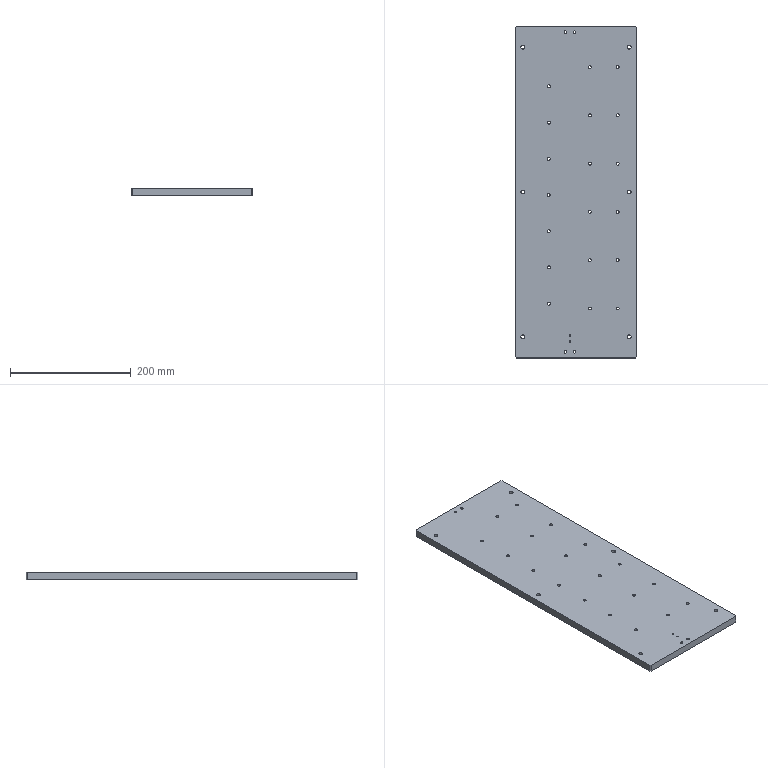Part | STEP file | ASND-0110-Body 1-8 | 1 solid | 90 faces | box 202 x 550 x 12 mm | volume 1322271 mm3 | cylinder 74 | plane 16 | commonest cylinder face diameters 4.917 x38 6.5 x12 12 x12 4.134 x8 2.459 x4